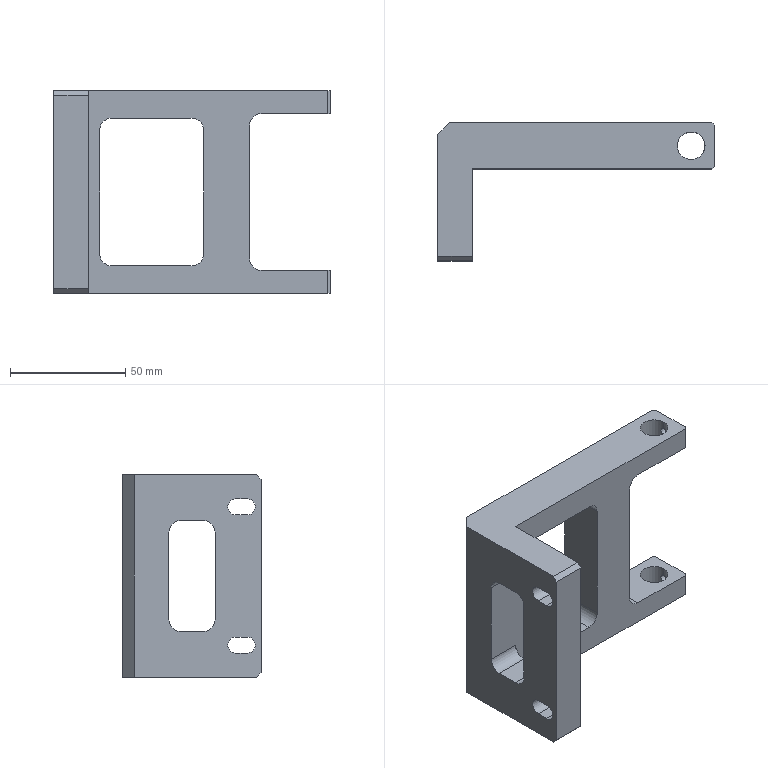Part | SolidWorks | features ICE 4, Chamfer 3, Extrusion 1, Fillet 1, HoleWzd 1 | 1 solid | 52 faces | box 120 x 60 x 88 mm | volume 139650 mm3 | plane 30 | cylinder 22 | commonest cylinder face diameters 10 x10 3.3 x4 7 x4 12 x4